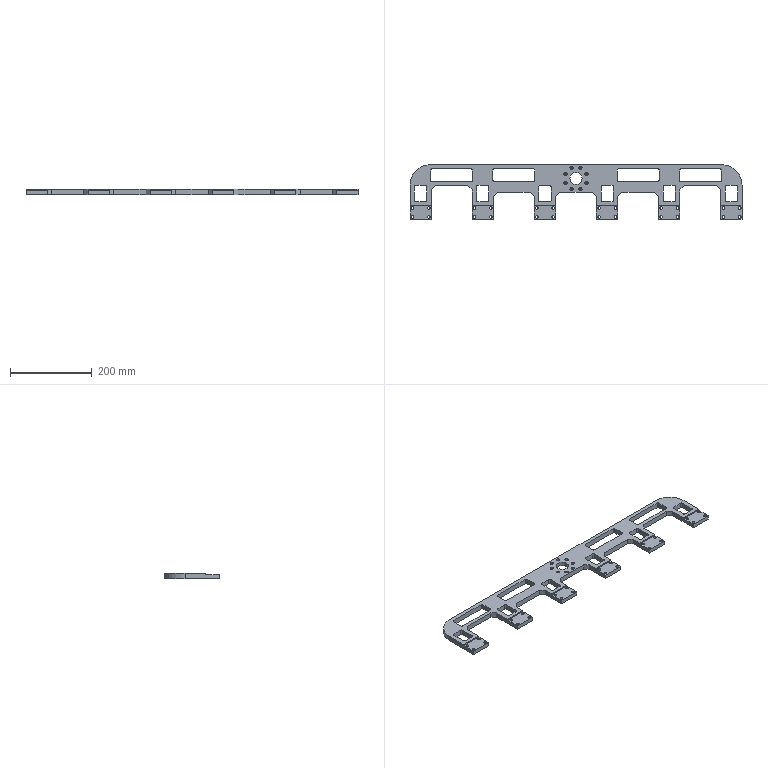NC program | NX | posted with a generic post | part box 813.6 x 134 x 13 mm
Lines 12952 to 13853 of 13853:
(PLANAR_MILL_COPY_1 , TOOL : D6A45)
N25842 T07 M6
N25844 G54
N25846 G17 G0 G90 X-393.7 Y-2.73 S9500 M3
N25848 G43 Z30. H7
N25850 Z0.
N25852 G94 G1 Z-1. F1400.
N25854 X-394.4 Y-3.134
N25856 G3 X-394.9 Y-4. R1.
N25858 G1 Y-21.
N25860 G3 X-392.8 Y-23.1 R2.1
N25862 G1 X-368.8
N25864 G3 X-366.7 Y-21. R2.1
N25866 G1 Y13.
N25868 G3 X-368.8 Y15.1 R2.1
N25870 G1 X-392.8
N25872 G3 X-394.9 Y13. R2.1
N25874 G1 Y-4.
N25876 G3 X-394.4 Y-4.866 R1.
N25878 G1 X-393.7 Y-5.27
N25880 Z0.
N25882 G0 Z30.
N25884 X-303.53 Y54.9
N25886 Z0.
N25888 G1 Z-1.
N25890 X-303.934 Y55.6
N25892 G3 X-304.8 Y56.1 R1.
N25894 G1 X-352.8
N25896 G3 X-354.9 Y54. R2.1
N25898 G1 Y28.
N25900 G3 X-352.8 Y25.9 R2.1
N25902 G1 X-256.8
N25904 G3 X-254.7 Y28. R2.1
N25906 G1 Y54.
N25908 G3 X-256.8 Y56.1 R2.1
N25910 G1 X-304.8
N25912 G3 X-305.666 Y55.6 R1.
N25914 G1 X-306.07 Y54.9
N25916 Z0.
N25918 G0 Z30.
N25920 X-241.3 Y-2.73
N25922 Z0.
N25924 G1 Z-1.
N25926 X-242. Y-3.134
N25928 G3 X-242.5 Y-4. R1.
N25930 G1 Y-21.
N25932 G3 X-240.4 Y-23.1 R2.1
N25934 G1 X-216.4
N25936 G3 X-214.3 Y-21. R2.1
N25938 G1 Y13.
N25940 G3 X-216.4 Y15.1 R2.1
N25942 G1 X-240.4
N25944 G3 X-242.5 Y13. R2.1
N25946 G1 Y-4.
N25948 G3 X-242. Y-4.866 R1.
N25950 G1 X-241.3 Y-5.27
N25952 Z0.
N25954 G0 Z30.
N25956 X-151.13 Y54.9
N25958 Z0.
N25960 G1 Z-1.
N25962 X-151.534 Y55.6
N25964 G3 X-152.4 Y56.1 R1.
N25966 G1 X-200.4
N25968 G3 X-202.5 Y54. R2.1
N25970 G1 Y28.
N25972 G3 X-200.4 Y25.9 R2.1
N25974 G1 X-104.4
N25976 G3 X-102.3 Y28. R2.1
N25978 G1 Y54.
N25980 G3 X-104.4 Y56.1 R2.1
N25982 G1 X-152.4
N25984 G3 X-153.266 Y55.6 R1.
N25986 G1 X-153.67 Y54.9
N25988 Z0.
N25990 G0 Z30.
N25992 X-88.9 Y-2.73
N25994 Z0.
N25996 G1 Z-1.
N25998 X-89.6 Y-3.134
N26000 G3 X-90.1 Y-4. R1.
N26002 G1 Y-21.
N26004 G3 X-88. Y-23.1 R2.1
N26006 G1 X-64.
N26008 G3 X-61.9 Y-21. R2.1
N26010 G1 Y13.
N26012 G3 X-64. Y15.1 R2.1
N26014 G1 X-88.
N26016 G3 X-90.1 Y13. R2.1
N26018 G1 Y-4.
N26020 G3 X-89.6 Y-4.866 R1.
N26022 G1 X-88.9 Y-5.27
N26024 Z0.
N26026 G0 Z30.
N26028 X-25.268 Y24.087
N26030 Z0.
N26032 G1 Z-1.
N26034 X-25.003 Y24.885
N26036 G3 X-25.869 Y25.385 R1.
N26038 X-28.969 Y22.285 R3.1
N26040 X-25.869 Y25.385 R-3.1
N26042 X-26.735 Y24.885 R1.
N26044 G1 X-26.469 Y24.087
N26046 Z0.
N26048 G0 Z30.
N26050 X-25.268 Y45.518
N26052 Z0.
N26054 G1 Z-1.
N26056 X-25.003 Y46.315
N26058 G3 X-25.869 Y46.815 R1.
N26060 X-28.969 Y43.715 R3.1
N26062 X-25.869 Y46.815 R-3.1
N26064 X-26.735 Y46.315 R1.
N26066 G1 X-26.469 Y45.518
N26068 Z0.
N26070 G0 Z30.
N26072 X-10.115 Y60.671
N26074 Z0.
N26076 G1 Z-1.
N26078 X-9.849 Y61.469
N26080 G3 X-10.715 Y61.969 R1.
N26082 X-13.815 Y58.869 R3.1
N26084 X-10.715 Y61.969 R-3.1
N26086 X-11.581 Y61.469 R1.
N26088 G1 X-11.316 Y60.671
N26090 Z0.
N26092 G0 Z30.
N26094 X11.316
N26096 Z0.
N26098 G1 Z-1.
N26100 X11.581 Y61.469
N26102 G3 X10.715 Y61.969 R1.
N26104 X7.615 Y58.869 R3.1
N26106 X10.715 Y61.969 R-3.1
N26108 X9.849 Y61.469 R1.
N26110 G1 X10.115 Y60.671
N26112 Z0.
N26114 G0 Z30.
N26116 X26.469 Y45.518
N26118 Z0.
N26120 G1 Z-1.
N26122 X26.735 Y46.315
N26124 G3 X25.869 Y46.815 R1.
N26126 X22.769 Y43.715 R3.1
N26128 X25.869 Y46.815 R-3.1
N26130 X25.003 Y46.315 R1.
N26132 G1 X25.268 Y45.518
N26134 Z0.
N26136 G0 Z30.
N26138 X26.469 Y24.087
N26140 Z0.
N26142 G1 Z-1.
N26144 X26.735 Y24.885
N26146 G3 X25.869 Y25.385 R1.
N26148 X22.769 Y22.285 R3.1
N26150 X25.869 Y25.385 R-3.1
N26152 X25.003 Y24.885 R1.
N26154 G1 X25.268 Y24.087
N26156 Z0.
N26158 G0 Z30.
N26160 X1.309 Y45.833
N26162 Z0.
N26164 G1 Z-1.
N26166 X0.866 Y46.6
N26168 G3 X0. Y47.1 R1.
N26170 X-14.1 Y33. R14.1
N26172 X0. Y47.1 R-14.1
N26174 X-0.866 Y46.6 R1.
N26176 G1 X-1.309 Y45.833
N26178 Z0.
N26180 G0 Z30.
N26182 X-11.316 Y5.329
N26184 Z0.
N26186 G1 Z-1.
N26188 X-11.581 Y4.531
N26190 G3 X-10.715 Y4.031 R1.
N26192 X-7.615 Y7.131 R3.1
N26194 X-10.715 Y4.031 R-3.1
N26196 X-9.849 Y4.531 R1.
N26198 G1 X-10.115 Y5.329
N26200 Z0.
N26202 G0 Z30.
N26204 X10.115
N26206 Z0.
N26208 G1 Z-1.
N26210 X9.849 Y4.531
N26212 G3 X10.715 Y4.031 R1.
N26214 X13.815 Y7.131 R3.1
N26216 X10.715 Y4.031 R-3.1
N26218 X11.581 Y4.531 R1.
N26220 G1 X11.316 Y5.329
N26222 Z0.
N26224 G0 Z30.
N26226 X-1.27 Y69.1
N26228 Z0.
N26230 G1 Z-1.
N26232 X-0.866 Y68.4
N26234 G3 X0. Y67.9 R1.
N26236 G1 X356.8
N26238 G2 X407.7 Y17. R50.9
N26240 G1 Y-33.3
N26242 G2 X406.7 Y-34.3 R1.
N26244 G1 X354.9
N26246 G2 X353.9 Y-33.3 R1.
N26248 G1 Y4.627
N26250 X344.427 Y14.1
N26252 X265.173
N26254 X255.7 Y4.627
N26256 Y-33.3
N26258 G2 X254.7 Y-34.3 R1.
N26260 G1 X202.5
N26262 G2 X201.5 Y-33.3 R1.
N26264 G1 Y-11.323
N26266 X192.027 Y-1.85
N26268 X112.773
N26270 X103.3 Y-11.323
N26272 Y-33.3
N26274 G2 X102.3 Y-34.3 R1.
N26276 G1 X50.1
N26278 G2 X49.1 Y-33.3 R1.
N26280 G1 Y-11.323
N26282 X39.627 Y-1.85
N26284 X-39.627
N26286 X-49.1 Y-11.323
N26288 Y-33.3
N26290 G2 X-50.1 Y-34.3 R1.
N26292 G1 X-102.3
N26294 G2 X-103.3 Y-33.3 R1.
N26296 G1 Y-11.323
N26298 X-112.773 Y-1.85
N26300 X-192.027
N26302 X-201.5 Y-11.323
N26304 Y-33.3
N26306 G2 X-202.5 Y-34.3 R1.
N26308 G1 X-254.7
N26310 G2 X-255.7 Y-33.3 R1.
N26312 G1 Y4.627
N26314 X-265.173 Y14.1
N26316 X-344.427
N26318 X-353.9 Y4.627
N26320 Y-33.3
N26322 G2 X-354.9 Y-34.3 R1.
N26324 G1 X-406.7
N26326 G2 X-407.7 Y-33.3 R1.
N26328 G1 Y17.
N26330 G2 X-356.8 Y67.9 R50.9
N26332 G1 X0.
N26334 G3 X0.866 Y68.4 R1.
N26336 G1 X1.27 Y69.1
N26338 Z0.
N26340 G0 Z30.
N26342 X63.5 Y-2.73
N26344 Z0.
N26346 G1 Z-1.
N26348 X62.8 Y-3.134
N26350 G3 X62.3 Y-4. R1.
N26352 G1 Y-21.
N26354 G3 X64.4 Y-23.1 R2.1
N26356 G1 X88.4
N26358 G3 X90.5 Y-21. R2.1
N26360 G1 Y13.
N26362 G3 X88.4 Y15.1 R2.1
N26364 G1 X64.4
N26366 G3 X62.3 Y13. R2.1
N26368 G1 Y-4.
N26370 G3 X62.8 Y-4.866 R1.
N26372 G1 X63.5 Y-5.27
N26374 Z0.
N26376 G0 Z30.
N26378 X153.67 Y54.9
N26380 Z0.
N26382 G1 Z-1.
N26384 X153.266 Y55.6
N26386 G3 X152.4 Y56.1 R1.
N26388 G1 X104.4
N26390 G3 X102.3 Y54. R2.1
N26392 G1 Y28.
N26394 G3 X104.4 Y25.9 R2.1
N26396 G1 X200.4
N26398 G3 X202.5 Y28. R2.1
N26400 G1 Y54.
N26402 G3 X200.4 Y56.1 R2.1
N26404 G1 X152.4
N26406 G3 X151.534 Y55.6 R1.
N26408 G1 X151.13 Y54.9
N26410 Z0.
N26412 G0 Z30.
N26414 X215.9 Y-2.73
N26416 Z0.
N26418 G1 Z-1.
N26420 X215.2 Y-3.134
N26422 G3 X214.7 Y-4. R1.
N26424 G1 Y-21.
N26426 G3 X216.8 Y-23.1 R2.1
N26428 G1 X240.8
N26430 G3 X242.9 Y-21. R2.1
N26432 G1 Y13.
N26434 G3 X240.8 Y15.1 R2.1
N26436 G1 X216.8
N26438 G3 X214.7 Y13. R2.1
N26440 G1 Y-4.
N26442 G3 X215.2 Y-4.866 R1.
N26444 G1 X215.9 Y-5.27
N26446 Z0.
N26448 G0 Z30.
N26450 X306.07 Y54.9
N26452 Z0.
N26454 G1 Z-1.
N26456 X305.666 Y55.6
N26458 G3 X304.8 Y56.1 R1.
N26460 G1 X256.8
N26462 G3 X254.7 Y54. R2.1
N26464 G1 Y28.
N26466 G3 X256.8 Y25.9 R2.1
N26468 G1 X352.8
N26470 G3 X354.9 Y28. R2.1
N26472 G1 Y54.
N26474 G3 X352.8 Y56.1 R2.1
N26476 G1 X304.8
N26478 G3 X303.934 Y55.6 R1.
N26480 G1 X303.53 Y54.9
N26482 Z0.
N26484 G0 Z30.
N26486 X394.1 Y-5.27
N26488 Z0.
N26490 G1 Z-1.
N26492 X394.8 Y-4.866
N26494 G3 X395.3 Y-4. R1.
N26496 G1 Y13.
N26498 G3 X393.2 Y15.1 R2.1
N26500 G1 X369.2
N26502 G3 X367.1 Y13. R2.1
N26504 G1 Y-21.
N26506 G3 X369.2 Y-23.1 R2.1
N26508 G1 X393.2
N26510 G3 X395.3 Y-21. R2.1
N26512 G1 Y-4.
N26514 G3 X394.8 Y-3.134 R1.
N26516 G1 X394.1 Y-2.73
N26518 Z0.
N26520 G0 Z30.
(PLANAR_MILL_COPY_1_COPY , TOOL : D6A45)
N26522 X400.712 Y-62.242
N26524 Z-3.
N26526 G1 Z-4.
N26528 X400.334 Y-63.05
N26530 G3 X401.2 Y-63.55 R1.
N26532 X403.55 Y-61.2 R2.35
N26534 X401.2 Y-63.55 R-2.35
N26536 X402.066 Y-63.05 R1.
N26538 G1 X401.688 Y-62.242
N26540 Z-3.
N26542 G0 Z30.
N26544 X401.193 Y-38.1
N26546 Z-3.
N26548 G1 Z-4.
N26550 Y-37.056
N26552 G3 X400.718 Y-36.9 R0.5
N26554 X401.682 Y-36.9 R-2.35
N26556 X401.207 Y-37.056 R0.5
N26558 G1 Y-38.1
N26560 Z-3.
N26562 G0 Z30.
N26564 X361.193
N26566 Z-3.
N26568 G1 Z-4.
N26570 Y-37.056
N26572 G3 X360.718 Y-36.9 R0.5
N26574 X361.682 Y-36.9 R-2.35
N26576 X361.207 Y-37.056 R0.5
N26578 G1 Y-38.1
N26580 Z-3.
N26582 G0 Z30.
N26584 X360.712 Y-62.242
N26586 Z-3.
N26588 G1 Z-4.
N26590 X360.334 Y-63.05
N26592 G3 X361.2 Y-63.55 R1.
N26594 X363.55 Y-61.2 R2.35
N26596 X361.2 Y-63.55 R-2.35
N26598 X362.066 Y-63.05 R1.
N26600 G1 X361.688 Y-62.242
N26602 Z-3.
N26604 G0 Z30.
N26606 X248.312
N26608 Z-3.
N26610 G1 Z-4.
N26612 X247.934 Y-63.05
N26614 G3 X248.8 Y-63.55 R1.
N26616 X251.15 Y-61.2 R2.35
N26618 X248.8 Y-63.55 R-2.35
N26620 X249.666 Y-63.05 R1.
N26622 G1 X249.288 Y-62.242
N26624 Z-3.
N26626 G0 Z30.
N26628 X248.793 Y-38.1
N26630 Z-3.
N26632 G1 Z-4.
N26634 Y-37.056
N26636 G3 X248.318 Y-36.9 R0.5
N26638 X249.282 Y-36.9 R-2.35
N26640 X248.807 Y-37.056 R0.5
N26642 G1 Y-38.1
N26644 Z-3.
N26646 G0 Z30.
N26648 X208.793
N26650 Z-3.
N26652 G1 Z-4.
N26654 Y-37.056
N26656 G3 X208.318 Y-36.9 R0.5
N26658 X209.282 Y-36.9 R-2.35
N26660 X208.807 Y-37.056 R0.5
N26662 G1 Y-38.1
N26664 Z-3.
N26666 G0 Z30.
N26668 X208.312 Y-62.242
N26670 Z-3.
N26672 G1 Z-4.
N26674 X207.934 Y-63.05
N26676 G3 X208.8 Y-63.55 R1.
N26678 X211.15 Y-61.2 R2.35
N26680 X208.8 Y-63.55 R-2.35
N26682 X209.666 Y-63.05 R1.
N26684 G1 X209.288 Y-62.242
N26686 Z-3.
N26688 G0 Z30.
N26690 X95.912
N26692 Z-3.
N26694 G1 Z-4.
N26696 X95.534 Y-63.05
N26698 G3 X96.4 Y-63.55 R1.
N26700 X98.75 Y-61.2 R2.35
N26702 X96.4 Y-63.55 R-2.35
N26704 X97.266 Y-63.05 R1.
N26706 G1 X96.888 Y-62.242
N26708 Z-3.
N26710 G0 Z30.
N26712 X96.393 Y-38.1
N26714 Z-3.
N26716 G1 Z-4.
N26718 Y-37.056
N26720 G3 X95.918 Y-36.9 R0.5
N26722 X96.882 Y-36.9 R-2.35
N26724 X96.407 Y-37.056 R0.5
N26726 G1 Y-38.1
N26728 Z-3.
N26730 G0 Z30.
N26732 X56.393
N26734 Z-3.
N26736 G1 Z-4.
N26738 Y-37.056
N26740 G3 X55.918 Y-36.9 R0.5
N26742 X56.882 Y-36.9 R-2.35
N26744 X56.407 Y-37.056 R0.5
N26746 G1 Y-38.1
N26748 Z-3.
N26750 G0 Z30.
N26752 X55.912 Y-62.242
N26754 Z-3.
N26756 G1 Z-4.
N26758 X55.534 Y-63.05
N26760 G3 X56.4 Y-63.55 R1.
N26762 X58.75 Y-61.2 R2.35
N26764 X56.4 Y-63.55 R-2.35
N26766 X57.266 Y-63.05 R1.
N26768 G1 X56.888 Y-62.242
N26770 Z-3.
N26772 G0 Z30.
N26774 X104.713 Y-37.492
N26776 Z-3.
N26778 G1 Z-4.
N26780 X104.265 Y-37.043
N26782 G3 X103.3 Y-36.782 R1.
N26784 G1 Y-66.9
N26786 G2 X102.3 Y-67.9 R1.
N26788 G1 X50.1
N26790 G2 X49.1 Y-66.9 R1.
N26792 G1 Y-36.782
N26794 G3 X48.135 Y-37.043 R1.
N26796 G1 X47.687 Y-37.492
N26798 Z-3.
N26800 G0 Z30.
N26802 X-47.687
N26804 Z-3.
N26806 G1 Z-4.
N26808 X-48.135 Y-37.043
N26810 G3 X-49.1 Y-36.782 R1.
N26812 G1 Y-66.9
N26814 G2 X-50.1 Y-67.9 R1.
N26816 G1 X-102.3
N26818 G2 X-103.3 Y-66.9 R1.
N26820 G1 Y-36.782
N26822 G3 X-104.265 Y-37.043 R1.
N26824 G1 X-104.713 Y-37.492
N26826 Z-3.
N26828 G0 Z30.
N26830 X-200.087
N26832 Z-3.
N26834 G1 Z-4.
N26836 X-200.535 Y-37.043
N26838 G3 X-201.5 Y-36.782 R1.
N26840 G1 Y-66.9
N26842 G2 X-202.5 Y-67.9 R1.
N26844 G1 X-254.7
N26846 G2 X-255.7 Y-66.9 R1.
N26848 G1 Y-36.782
N26850 G3 X-256.665 Y-37.043 R1.
N26852 G1 X-257.113 Y-37.492
N26854 Z-3.
N26856 G0 Z30.
N26858 X-352.487
N26860 Z-3.
N26862 G1 Z-4.
N26864 X-352.935 Y-37.043
N26866 G3 X-353.9 Y-36.782 R1.
N26868 G1 Y-66.9
N26870 G2 X-354.9 Y-67.9 R1.
N26872 G1 X-406.7
N26874 G2 X-407.7 Y-66.9 R1.
N26876 G1 Y-36.782
N26878 G3 X-408.665 Y-37.043 R1.
N26880 G1 X-409.113 Y-37.492
N26882 Z-3.
N26884 G0 Z30.
N26886 X409.113
N26888 Z-3.
N26890 G1 Z-4.
N26892 X408.665 Y-37.043
N26894 G3 X407.7 Y-36.782 R1.
N26896 G1 Y-66.9
N26898 G2 X406.7 Y-67.9 R1.
N26900 G1 X354.9
N26902 G2 X353.9 Y-66.9 R1.
N26904 G1 Y-36.782
N26906 G3 X352.935 Y-37.043 R1.
N26908 G1 X352.487 Y-37.492
N26910 Z-3.
N26912 G0 Z30.
N26914 X257.113
N26916 Z-3.
N26918 G1 Z-4.
N26920 X256.665 Y-37.043
N26922 G3 X255.7 Y-36.782 R1.
N26924 G1 Y-66.9
N26926 G2 X254.7 Y-67.9 R1.
N26928 G1 X202.5
N26930 G2 X201.5 Y-66.9 R1.
N26932 G1 Y-36.782
N26934 G3 X200.535 Y-37.043 R1.
N26936 G1 X200.087 Y-37.492
N26938 Z-3.
N26940 G0 Z30.
N26942 X-56.488 Y-62.242
N26944 Z-3.
N26946 G1 Z-4.
N26948 X-56.866 Y-63.05
N26950 G3 X-56. Y-63.55 R1.
N26952 X-53.65 Y-61.2 R2.35
N26954 X-56. Y-63.55 R-2.35
N26956 X-55.134 Y-63.05 R1.
N26958 G1 X-55.512 Y-62.242
N26960 Z-3.
N26962 G0 Z30.
N26964 X-56.007 Y-38.1
N26966 Z-3.
N26968 G1 Z-4.
N26970 Y-37.056
N26972 G3 X-56.482 Y-36.9 R0.5
N26974 X-55.518 Y-36.9 R-2.35
N26976 X-55.993 Y-37.056 R0.5
N26978 G1 Y-38.1
N26980 Z-3.
N26982 G0 Z30.
N26984 X-96.007
N26986 Z-3.
N26988 G1 Z-4.
N26990 Y-37.056
N26992 G3 X-96.482 Y-36.9 R0.5
N26994 X-95.518 Y-36.9 R-2.35
N26996 X-95.993 Y-37.056 R0.5
N26998 G1 Y-38.1
N27000 Z-3.
N27002 G0 Z30.
N27004 X-96.488 Y-62.242
N27006 Z-3.
N27008 G1 Z-4.
N27010 X-96.866 Y-63.05
N27012 G3 X-96. Y-63.55 R1.
N27014 X-93.65 Y-61.2 R2.35
N27016 X-96. Y-63.55 R-2.35
N27018 X-95.134 Y-63.05 R1.
N27020 G1 X-95.512 Y-62.242
N27022 Z-3.
N27024 G0 Z30.
N27026 X-208.888
N27028 Z-3.
N27030 G1 Z-4.
N27032 X-209.266 Y-63.05
N27034 G3 X-208.4 Y-63.55 R1.
N27036 X-206.05 Y-61.2 R2.35
N27038 X-208.4 Y-63.55 R-2.35
N27040 X-207.534 Y-63.05 R1.
N27042 G1 X-207.912 Y-62.242
N27044 Z-3.
N27046 G0 Z30.
N27048 X-208.407 Y-38.1
N27050 Z-3.
N27052 G1 Z-4.
N27054 Y-37.056
N27056 G3 X-208.882 Y-36.9 R0.5
N27058 X-207.918 Y-36.9 R-2.35
N27060 X-208.393 Y-37.056 R0.5
N27062 G1 Y-38.1
N27064 Z-3.
N27066 G0 Z30.
N27068 X-248.407
N27070 Z-3.
N27072 G1 Z-4.
N27074 Y-37.056
N27076 G3 X-248.882 Y-36.9 R0.5
N27078 X-247.918 Y-36.9 R-2.35
N27080 X-248.393 Y-37.056 R0.5
N27082 G1 Y-38.1
N27084 Z-3.
N27086 G0 Z30.
N27088 X-248.888 Y-62.242
N27090 Z-3.
N27092 G1 Z-4.
N27094 X-249.266 Y-63.05
N27096 G3 X-248.4 Y-63.55 R1.
N27098 X-246.05 Y-61.2 R2.35
N27100 X-248.4 Y-63.55 R-2.35
N27102 X-247.534 Y-63.05 R1.
N27104 G1 X-247.912 Y-62.242
N27106 Z-3.
N27108 G0 Z30.
N27110 X-361.288
N27112 Z-3.
N27114 G1 Z-4.
N27116 X-361.666 Y-63.05
N27118 G3 X-360.8 Y-63.55 R1.
N27120 X-358.45 Y-61.2 R2.35
N27122 X-360.8 Y-63.55 R-2.35
N27124 X-359.934 Y-63.05 R1.
N27126 G1 X-360.312 Y-62.242
N27128 Z-3.
N27130 G0 Z30.
N27132 X-360.807 Y-38.1
N27134 Z-3.
N27136 G1 Z-4.
N27138 Y-37.056
N27140 G3 X-361.282 Y-36.9 R0.5
N27142 X-360.318 Y-36.9 R-2.35
N27144 X-360.793 Y-37.056 R0.5
N27146 G1 Y-38.1
N27148 Z-3.
N27150 G0 Z30.
N27152 X-400.807
N27154 Z-3.
N27156 G1 Z-4.
N27158 Y-37.056
N27160 G3 X-401.282 Y-36.9 R0.5
N27162 X-400.318 Y-36.9 R-2.35
N27164 X-400.793 Y-37.056 R0.5
N27166 G1 Y-38.1
N27168 Z-3.
N27170 G0 Z30.
N27172 X-401.288 Y-62.242
N27174 Z-3.
N27176 G1 Z-4.
N27178 X-401.666 Y-63.05
N27180 G3 X-400.8 Y-63.55 R1.
N27182 X-398.45 Y-61.2 R2.35
N27184 X-400.8 Y-63.55 R-2.35
N27186 X-399.934 Y-63.05 R1.
N27188 G1 X-400.312 Y-62.242
N27190 Z-3.
N27192 G0 Z30.
N27194 M5
(ZLEVEL_PROFILE_COPY_3_COPY , TOOL : D10)
N27196 T10 M6
N27198 G54
N27200 G17 G0 G90 X-359.366 Y75.444 S9500 M3
N27202 G43 Z30. H10
N27204 Z-7.525
N27206 G94 G1 Z-12.525 F1000.
N27208 X-357.667 Y72.5
N27210 G3 X-356.801 Y72. R1.
N27212 G1 X356.8 F1200.
N27214 G2 X411.8 Y17. R55.
N27216 G1 Y-67.
N27218 G2 X406.8 Y-72. R5.
N27220 G1 X354.8
N27222 G2 X349.8 Y-67. R5.
N27224 G1 Y2.929
N27226 X342.729 Y10.
N27228 X266.871
N27230 X259.8 Y2.929
N27232 Y-67.
N27234 G2 X254.8 Y-72. R5.
N27236 G1 X202.4
N27238 G2 X197.4 Y-67. R5.
N27240 G1 Y-13.021
N27242 X190.329 Y-5.95
N27244 X114.471
N27246 X107.4 Y-13.021
N27248 Y-67.
N27250 G2 X102.4 Y-72. R5.
N27252 G1 X50.
N27254 G2 X45. Y-67. R5.
N27256 G1 Y-13.021
N27258 X37.929 Y-5.95
N27260 X-37.929
N27262 X-45. Y-13.021
N27264 Y-67.
N27266 G2 X-50. Y-72. R5.
N27268 G1 X-102.4
N27270 G2 X-107.4 Y-67. R5.
N27272 G1 Y-13.021
N27274 X-114.471 Y-5.95
N27276 X-190.329
N27278 X-197.4 Y-13.021
N27280 Y-67.
N27282 G2 X-202.4 Y-72. R5.
N27284 G1 X-254.8
N27286 G2 X-259.8 Y-67. R5.
N27288 G1 Y2.929
N27290 X-266.871 Y10.
N27292 X-342.729
N27294 X-349.8 Y2.929
N27296 Y-67.
N27298 G2 X-354.8 Y-72. R5.
N27300 G1 X-406.8
N27302 G2 X-411.8 Y-67. R5.
N27304 G1 Y17.006
N27306 G2 X-356.801 Y72. R55.
N27308 G1 X-356.59 Z-12.529
N27310 X-349.85 Z-12.646
N27312 X-349.639 Z-12.65
N27314 X356.8
N27316 G2 X411.8 Y17. R55.
N27318 G1 Y-67.
N27320 G2 X406.8 Y-72. R5.
N27322 G1 X354.8
N27324 G2 X349.8 Y-67. R5.
N27326 G1 Y2.929
N27328 X342.729 Y10.
N27330 X266.871
N27332 X259.8 Y2.929
N27334 Y-67.
N27336 G2 X254.8 Y-72. R5.
N27338 G1 X202.4
N27340 G2 X197.4 Y-67. R5.
N27342 G1 Y-13.021
N27344 X190.329 Y-5.95
N27346 X114.471
N27348 X107.4 Y-13.021
N27350 Y-67.
N27352 G2 X102.4 Y-72. R5.
N27354 G1 X50.
N27356 G2 X45. Y-67. R5.
N27358 G1 Y-13.021
N27360 X37.929 Y-5.95
N27362 X-37.929
N27364 X-45. Y-13.021
N27366 Y-67.
N27368 G2 X-50. Y-72. R5.
N27370 G1 X-102.4
N27372 G2 X-107.4 Y-67. R5.
N27374 G1 Y-13.021
N27376 X-114.471 Y-5.95
N27378 X-190.329
N27380 X-197.4 Y-13.021
N27382 Y-67.
N27384 G2 X-202.4 Y-72. R5.
N27386 G1 X-254.8
N27388 G2 X-259.8 Y-67. R5.
N27390 G1 Y2.929
N27392 X-266.871 Y10.
N27394 X-342.729
N27396 X-349.8 Y2.929
N27398 Y-67.
N27400 G2 X-354.8 Y-72. R5.
N27402 G1 X-406.8
N27404 G2 X-411.8 Y-67. R5.
N27406 G1 Y17.006
N27408 G2 X-356.801 Y72. R55.
N27410 G1 X-356.59 Z-12.654
N27412 X-349.85 Z-12.771
N27414 X-349.639 Z-12.775
N27416 X356.8
N27418 G2 X411.8 Y17. R55.
N27420 G1 Y-67.
N27422 G2 X406.8 Y-72. R5.
N27424 G1 X354.8
N27426 G2 X349.8 Y-67. R5.
N27428 G1 Y2.929
N27430 X342.729 Y10.
N27432 X266.871
N27434 X259.8 Y2.929
N27436 Y-67.
N27438 G2 X254.8 Y-72. R5.
N27440 G1 X202.4
N27442 G2 X197.4 Y-67. R5.
N27444 G1 Y-13.021
N27446 X190.329 Y-5.95
N27448 X114.471
N27450 X107.4 Y-13.021
N27452 Y-67.
N27454 G2 X102.4 Y-72. R5.
N27456 G1 X50.
N27458 G2 X45. Y-67. R5.
N27460 G1 Y-13.021
N27462 X37.929 Y-5.95
N27464 X-37.929
N27466 X-45. Y-13.021
N27468 Y-67.
N27470 G2 X-50. Y-72. R5.
N27472 G1 X-102.4
N27474 G2 X-107.4 Y-67. R5.
N27476 G1 Y-13.021
N27478 X-114.471 Y-5.95
N27480 X-190.329
N27482 X-197.4 Y-13.021
N27484 Y-67.
N27486 G2 X-202.4 Y-72. R5.
N27488 G1 X-254.8
N27490 G2 X-259.8 Y-67. R5.
N27492 G1 Y2.929
N27494 X-266.871 Y10.
N27496 X-342.729
N27498 X-349.8 Y2.929
N27500 Y-67.
N27502 G2 X-354.8 Y-72. R5.
N27504 G1 X-406.8
N27506 G2 X-411.8 Y-67. R5.
N27508 G1 Y17.006
N27510 G2 X-356.801 Y72. R55.
N27512 G1 X-356.59 Z-12.779
N27514 X-349.85 Z-12.896
N27516 X-349.639 Z-12.9
N27518 X356.8
N27520 G2 X411.8 Y17. R55.
N27522 G1 Y-67.
N27524 G2 X406.8 Y-72. R5.
N27526 G1 X354.8
N27528 G2 X349.8 Y-67. R5.
N27530 G1 Y2.929
N27532 X342.729 Y10.
N27534 X266.871
N27536 X259.8 Y2.929
N27538 Y-67.
N27540 G2 X254.8 Y-72. R5.
N27542 G1 X202.4
N27544 G2 X197.4 Y-67. R5.
N27546 G1 Y-13.021
N27548 X190.329 Y-5.95
N27550 X114.471
N27552 X107.4 Y-13.021
N27554 Y-67.
N27556 G2 X102.4 Y-72. R5.
N27558 G1 X50.
N27560 G2 X45. Y-67. R5.
N27562 G1 Y-13.021
N27564 X37.929 Y-5.95
N27566 X-37.929
N27568 X-45. Y-13.021
N27570 Y-67.
N27572 G2 X-50. Y-72. R5.
N27574 G1 X-102.4
N27576 G2 X-107.4 Y-67. R5.
N27578 G1 Y-13.021
N27580 X-114.471 Y-5.95
N27582 X-190.329
N27584 X-197.4 Y-13.021
N27586 Y-67.
N27588 G2 X-202.4 Y-72. R5.
N27590 G1 X-254.8
N27592 G2 X-259.8 Y-67. R5.
N27594 G1 Y2.929
N27596 X-266.871 Y10.
N27598 X-342.729
N27600 X-349.8 Y2.929
N27602 Y-67.
N27604 G2 X-354.8 Y-72. R5.
N27606 G1 X-406.8
N27608 G2 X-411.8 Y-67. R5.
N27610 G1 Y17.006
N27612 G2 X-356.801 Y72. R55.
N27614 G1 X-349.639
N27616 G3 X-348.773 Y72.5 R1.
N27618 G1 X-347.041 Y75.5
N27620 Z-7.9
N27622 G0 Z30.
N27624 M5
N27626 M2